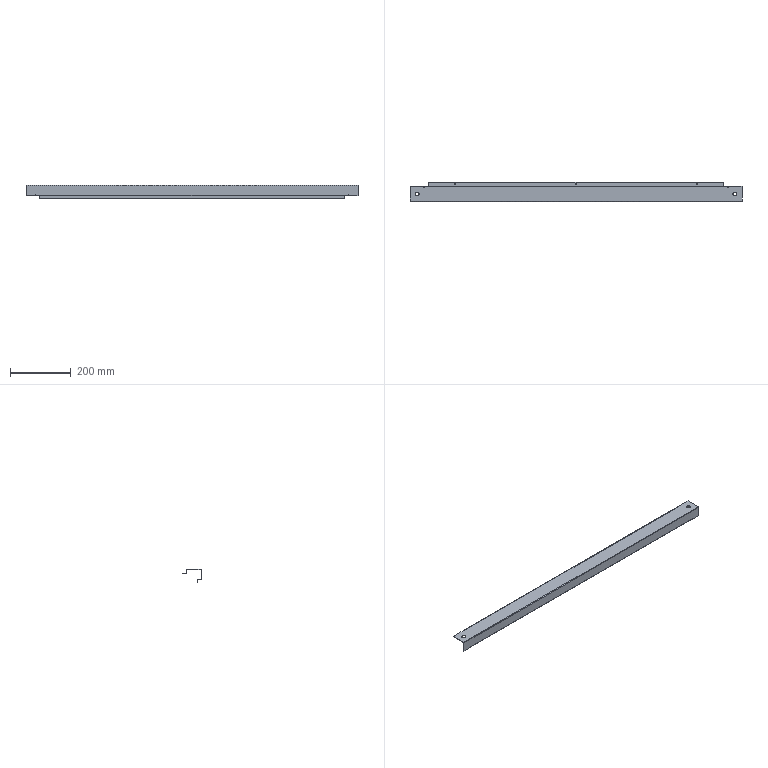Part | SolidWorks | features EdgeFlange 5, ICE 2, FlatPattern 1, SMBaseFlange 1, SheetMetal 1 | 1 solid | 88 faces | box 1097 x 63.5 x 45.5 mm | volume 210913 mm3 | plane 68 | cylinder 20 | commonest cylinder face diameters 5.1 x6 0.2 x5 3.2 x5 13 x4